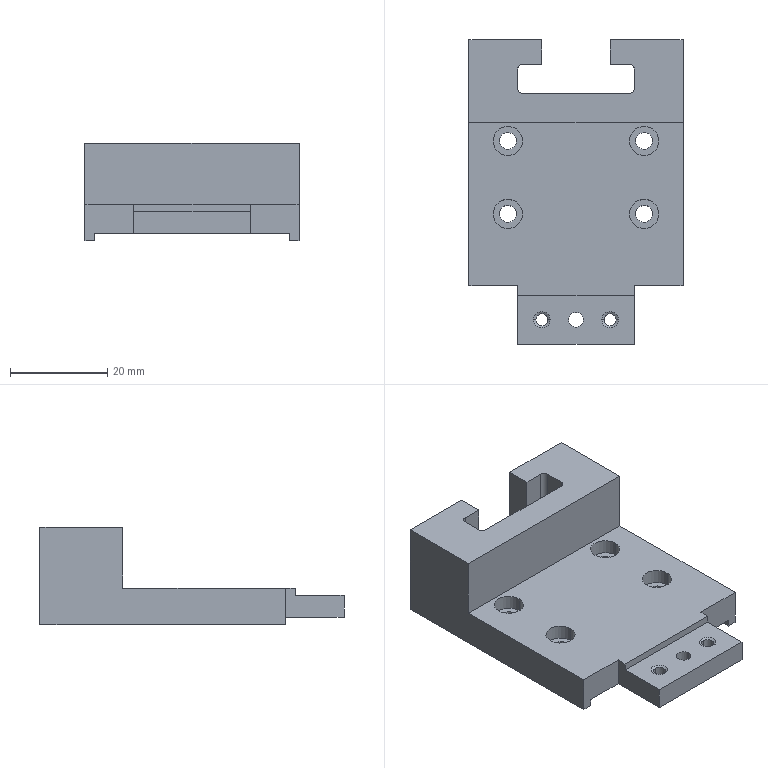Part | NX | 1 solid | 60 faces | box 44 x 62.5 x 20 mm | volume 19878 mm3 | plane 30 | cylinder 26 | cone 4 | commonest cylinder face diameters 3.5 x8 6 x8 2 x4 2.5 x4 3 x2